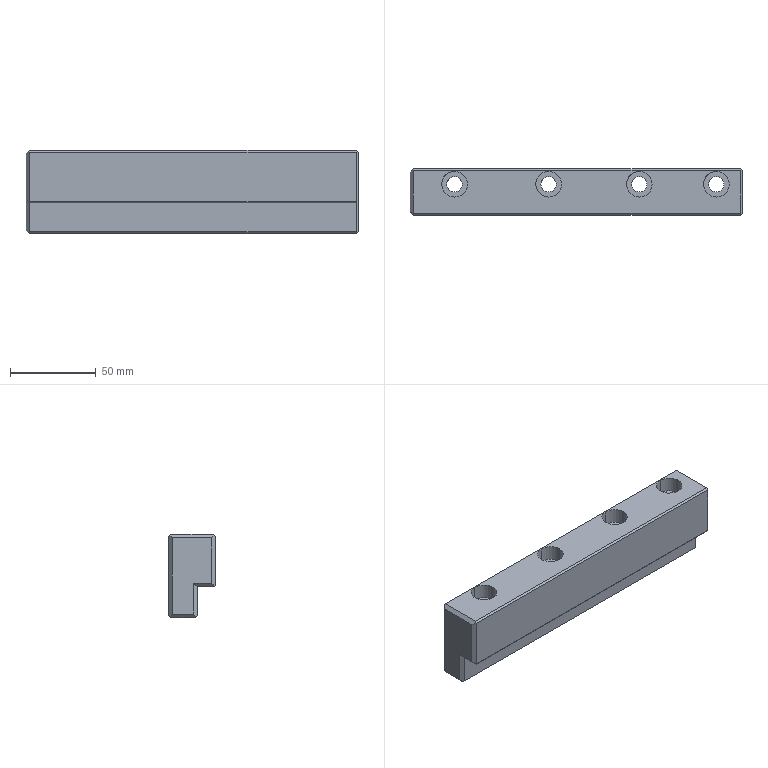Part | Creo | 1 solid | 45 faces | box 194 x 27 x 48.5 mm | volume 200192 mm3 | plane 29 | cylinder 16 | commonest cylinder face diameters 9 x8 15 x8
STEP:
#1=CARTESIAN_POINT('',(-122.,174.995,-41.));
#2=VERTEX_POINT('',#1);
#3=CARTESIAN_POINT('',(-122.,174.995,-12.));
#4=VERTEX_POINT('',#3);
#5=CARTESIAN_POINT('',(-122.,174.995,-41.));
#6=DIRECTION('',(0.,0.,1.));
#7=VECTOR('',#6,29.);
#8=LINE('',#5,#7);
#9=EDGE_CURVE('',#2,#4,#8,.T.);
#10=ORIENTED_EDGE('',*,*,#9,.F.);
#11=CARTESIAN_POINT('',(-313.,174.995,-41.));
#12=VERTEX_POINT('',#11);
#13=CARTESIAN_POINT('',(-313.,174.995,-41.));
#14=DIRECTION('',(1.,0.,0.));
#15=VECTOR('',#14,191.);
#16=LINE('',#13,#15);
#17=EDGE_CURVE('',#12,#2,#16,.T.);
#18=ORIENTED_EDGE('',*,*,#17,.F.);
#19=CARTESIAN_POINT('',(-313.,174.995,-12.));
#20=VERTEX_POINT('',#19);
#21=CARTESIAN_POINT('',(-313.,174.995,-12.));
#22=DIRECTION('',(0.,0.,-1.));
#23=VECTOR('',#22,29.);
#24=LINE('',#21,#23);
#25=EDGE_CURVE('',#20,#12,#24,.T.);
#26=ORIENTED_EDGE('',*,*,#25,.F.);
#27=CARTESIAN_POINT('',(-313.,174.995,-12.));
#28=DIRECTION('',(1.,0.,0.));
#29=VECTOR('',#28,191.);
#30=LINE('',#27,#29);
#31=EDGE_CURVE('',#20,#4,#30,.T.);
#32=ORIENTED_EDGE('',*,*,#31,.T.);
#33=EDGE_LOOP('',(#10,#18,#26,#32));
#34=FACE_OUTER_BOUND('',#33,.F.);
#35=CARTESIAN_POINT('',(-264.,174.995,-8.));
#36=DIRECTION('',(0.,-1.,0.));
#37=DIRECTION('',(0.,0.,1.));
#38=AXIS2_PLACEMENT_3D('',#35,#36,#37);
#39=PLANE('',#38);
#40=ADVANCED_FACE('',(#34),#39,.T.);
#41=CARTESIAN_POINT('',(-121.,175.995,-40.5));
#42=VERTEX_POINT('',#41);
#43=CARTESIAN_POINT('',(-121.,175.995,-12.));
#44=VERTEX_POINT('',#43);
#45=CARTESIAN_POINT('',(-121.,175.995,-40.5));
#46=DIRECTION('',(0.,0.,1.));
#47=VECTOR('',#46,28.5);
#48=LINE('',#45,#47);
#49=EDGE_CURVE('',#42,#44,#48,.T.);
#50=ORIENTED_EDGE('',*,*,#49,.F.);
#51=CARTESIAN_POINT('',(-121.75,175.245,-41.25));
#52=VERTEX_POINT('',#51);
#53=CARTESIAN_POINT('',(-121.,175.995,-40.5));
#54=DIRECTION('',(-0.5774,-0.5774,-0.5774));
#55=VECTOR('',#54,1.299);
#56=LINE('',#53,#55);
#57=EDGE_CURVE('',#42,#52,#56,.T.);
#58=ORIENTED_EDGE('',*,*,#57,.T.);
#59=CARTESIAN_POINT('',(-121.75,175.245,-41.25));
#60=DIRECTION('',(-0.5774,-0.5774,0.5774));
#61=VECTOR('',#60,0.433);
#62=LINE('',#59,#61);
#63=EDGE_CURVE('',#52,#2,#62,.T.);
#64=ORIENTED_EDGE('',*,*,#63,.T.);
#65=ORIENTED_EDGE('',*,*,#9,.T.);
#66=CARTESIAN_POINT('',(-121.5,175.495,-11.5));
#67=VERTEX_POINT('',#66);
#68=CARTESIAN_POINT('',(-122.,174.995,-12.));
#69=DIRECTION('',(0.5774,0.5774,0.5774));
#70=VECTOR('',#69,0.866);
#71=LINE('',#68,#70);
#72=EDGE_CURVE('',#4,#67,#71,.T.);
#73=ORIENTED_EDGE('',*,*,#72,.T.);
#74=CARTESIAN_POINT('',(-121.5,175.495,-11.5));
#75=DIRECTION('',(0.5774,0.5774,-0.5774));
#76=VECTOR('',#75,0.866);
#77=LINE('',#74,#76);
#78=EDGE_CURVE('',#67,#44,#77,.T.);
#79=ORIENTED_EDGE('',*,*,#78,.T.);
#80=EDGE_LOOP('',(#50,#58,#64,#65,#73,#79));
#81=FACE_OUTER_BOUND('',#80,.F.);
#82=CARTESIAN_POINT('',(-121.5,175.495,-25.75));
#83=DIRECTION('',(0.7071,-0.7071,0.));
#84=DIRECTION('',(0.7071,0.7071,0.));
#85=AXIS2_PLACEMENT_3D('',#82,#83,#84);
#86=PLANE('',#85);
#87=ADVANCED_FACE('',(#81),#86,.T.);
#88=CARTESIAN_POINT('',(-121.,200.995,-12.));
#89=VERTEX_POINT('',#88);
#90=CARTESIAN_POINT('',(-121.,200.995,-58.5));
#91=VERTEX_POINT('',#90);
#92=CARTESIAN_POINT('',(-121.,200.995,-12.));
#93=DIRECTION('',(0.,0.,-1.));
#94=VECTOR('',#93,46.5);
#95=LINE('',#92,#94);
#96=EDGE_CURVE('',#89,#91,#95,.T.);
#97=ORIENTED_EDGE('',*,*,#96,.T.);
#98=CARTESIAN_POINT('',(-121.,186.495,-58.5));
#99=VERTEX_POINT('',#98);
#100=CARTESIAN_POINT('',(-121.,200.995,-58.5));
#101=DIRECTION('',(0.,-1.,0.));
#102=VECTOR('',#101,14.5);
#103=LINE('',#100,#102);
#104=EDGE_CURVE('',#91,#99,#103,.T.);
#105=ORIENTED_EDGE('',*,*,#104,.T.);
#106=CARTESIAN_POINT('',(-121.,186.495,-40.5));
#107=VERTEX_POINT('',#106);
#108=CARTESIAN_POINT('',(-121.,186.495,-58.5));
#109=DIRECTION('',(0.,0.,1.));
#110=VECTOR('',#109,18.);
#111=LINE('',#108,#110);
#112=EDGE_CURVE('',#99,#107,#111,.T.);
#113=ORIENTED_EDGE('',*,*,#112,.T.);
#114=CARTESIAN_POINT('',(-121.,186.495,-40.5));
#115=DIRECTION('',(0.,-1.,0.));
#116=VECTOR('',#115,10.5);
#117=LINE('',#114,#116);
#118=EDGE_CURVE('',#107,#42,#117,.T.);
#119=ORIENTED_EDGE('',*,*,#118,.T.);
#120=ORIENTED_EDGE('',*,*,#49,.T.);
#121=CARTESIAN_POINT('',(-121.,175.995,-12.));
#122=DIRECTION('',(0.,1.,0.));
#123=VECTOR('',#122,25.);
#124=LINE('',#121,#123);
#125=EDGE_CURVE('',#44,#89,#124,.T.);
#126=ORIENTED_EDGE('',*,*,#125,.T.);
#127=EDGE_LOOP('',(#97,#105,#113,#119,#120,#126));
#128=FACE_OUTER_BOUND('',#127,.F.);
#129=CARTESIAN_POINT('',(-121.,183.495,-43.5));
#130=DIRECTION('',(1.,0.,0.));
#131=DIRECTION('',(0.,0.,-1.));
#132=AXIS2_PLACEMENT_3D('',#129,#130,#131);
#133=PLANE('',#132);
#134=ADVANCED_FACE('',(#128),#133,.T.);
#135=CARTESIAN_POINT('',(-122.,201.995,-12.));
#136=VERTEX_POINT('',#135);
#137=CARTESIAN_POINT('',(-122.,201.995,-58.5));
#138=VERTEX_POINT('',#137);
#139=CARTESIAN_POINT('',(-122.,201.995,-12.));
#140=DIRECTION('',(0.,0.,-1.));
#141=VECTOR('',#140,46.5);
#142=LINE('',#139,#141);
#143=EDGE_CURVE('',#136,#138,#142,.T.);
#144=ORIENTED_EDGE('',*,*,#143,.T.);
#145=CARTESIAN_POINT('',(-121.5,201.495,-59.));
#146=VERTEX_POINT('',#145);
#147=CARTESIAN_POINT('',(-121.5,201.495,-59.));
#148=DIRECTION('',(-0.5774,0.5774,0.5774));
#149=VECTOR('',#148,0.866);
#150=LINE('',#147,#149);
#151=EDGE_CURVE('',#146,#138,#150,.T.);
#152=ORIENTED_EDGE('',*,*,#151,.F.);
#153=CARTESIAN_POINT('',(-121.,200.995,-58.5));
#154=DIRECTION('',(-0.5774,0.5774,-0.5774));
#155=VECTOR('',#154,0.866);
#156=LINE('',#153,#155);
#157=EDGE_CURVE('',#91,#146,#156,.T.);
#158=ORIENTED_EDGE('',*,*,#157,.F.);
#159=ORIENTED_EDGE('',*,*,#96,.F.);
#160=CARTESIAN_POINT('',(-121.5,201.495,-11.5));
#161=VERTEX_POINT('',#160);
#162=CARTESIAN_POINT('',(-121.,200.995,-12.));
#163=DIRECTION('',(-0.5774,0.5774,0.5774));
#164=VECTOR('',#163,0.866);
#165=LINE('',#162,#164);
#166=EDGE_CURVE('',#89,#161,#165,.T.);
#167=ORIENTED_EDGE('',*,*,#166,.T.);
#168=CARTESIAN_POINT('',(-121.5,201.495,-11.5));
#169=DIRECTION('',(-0.5774,0.5774,-0.5774));
#170=VECTOR('',#169,0.866);
#171=LINE('',#168,#170);
#172=EDGE_CURVE('',#161,#136,#171,.T.);
#173=ORIENTED_EDGE('',*,*,#172,.T.);
#174=EDGE_LOOP('',(#144,#152,#158,#159,#167,#173));
#175=FACE_OUTER_BOUND('',#174,.F.);
#176=CARTESIAN_POINT('',(-121.5,201.495,-33.75));
#177=DIRECTION('',(0.7071,0.7071,0.));
#178=DIRECTION('',(0.7071,-0.7071,0.));
#179=AXIS2_PLACEMENT_3D('',#176,#177,#178);
#180=PLANE('',#179);
#181=ADVANCED_FACE('',(#175),#180,.T.);
#182=CARTESIAN_POINT('',(-313.,201.995,-58.5));
#183=VERTEX_POINT('',#182);
#184=CARTESIAN_POINT('',(-313.,201.995,-12.));
#185=VERTEX_POINT('',#184);
#186=CARTESIAN_POINT('',(-313.,201.995,-58.5));
#187=DIRECTION('',(0.,0.,1.));
#188=VECTOR('',#187,46.5);
#189=LINE('',#186,#188);
#190=EDGE_CURVE('',#183,#185,#189,.T.);
#191=ORIENTED_EDGE('',*,*,#190,.F.);
#192=CARTESIAN_POINT('',(-313.,201.995,-58.5));
#193=DIRECTION('',(1.,0.,0.));
#194=VECTOR('',#193,191.);
#195=LINE('',#192,#194);
#196=EDGE_CURVE('',#183,#138,#195,.T.);
#197=ORIENTED_EDGE('',*,*,#196,.T.);
#198=ORIENTED_EDGE('',*,*,#143,.F.);
#199=CARTESIAN_POINT('',(-122.,201.995,-12.));
#200=DIRECTION('',(-1.,0.,0.));
#201=VECTOR('',#200,191.);
#202=LINE('',#199,#201);
#203=EDGE_CURVE('',#136,#185,#202,.T.);
#204=ORIENTED_EDGE('',*,*,#203,.T.);
#205=EDGE_LOOP('',(#191,#197,#198,#204));
#206=FACE_OUTER_BOUND('',#205,.F.);
#207=CARTESIAN_POINT('',(-264.,201.995,-59.5));
#208=DIRECTION('',(0.,1.,0.));
#209=DIRECTION('',(0.,0.,-1.));
#210=AXIS2_PLACEMENT_3D('',#207,#208,#209);
#211=PLANE('',#210);
#212=ADVANCED_FACE('',(#206),#211,.T.);
#213=CARTESIAN_POINT('',(-315.,199.995,-57.5));
#214=VERTEX_POINT('',#213);
#215=CARTESIAN_POINT('',(-315.,199.995,-13.));
#216=VERTEX_POINT('',#215);
#217=CARTESIAN_POINT('',(-315.,199.995,-57.5));
#218=DIRECTION('',(0.,0.,1.));
#219=VECTOR('',#218,44.5);
#220=LINE('',#217,#219);
#221=EDGE_CURVE('',#214,#216,#220,.T.);
#222=ORIENTED_EDGE('',*,*,#221,.F.);
#223=CARTESIAN_POINT('',(-313.5,201.495,-59.));
#224=VERTEX_POINT('',#223);
#225=CARTESIAN_POINT('',(-313.5,201.495,-59.));
#226=DIRECTION('',(-0.5774,-0.5774,0.5774));
#227=VECTOR('',#226,2.598);
#228=LINE('',#225,#227);
#229=EDGE_CURVE('',#224,#214,#228,.T.);
#230=ORIENTED_EDGE('',*,*,#229,.F.);
#231=CARTESIAN_POINT('',(-313.,201.995,-58.5));
#232=DIRECTION('',(-0.5774,-0.5774,-0.5774));
#233=VECTOR('',#232,0.866);
#234=LINE('',#231,#233);
#235=EDGE_CURVE('',#183,#224,#234,.T.);
#236=ORIENTED_EDGE('',*,*,#235,.F.);
#237=ORIENTED_EDGE('',*,*,#190,.T.);
#238=CARTESIAN_POINT('',(-313.5,201.495,-11.5));
#239=VERTEX_POINT('',#238);
#240=CARTESIAN_POINT('',(-313.,201.995,-12.));
#241=DIRECTION('',(-0.5774,-0.5774,0.5774));
#242=VECTOR('',#241,0.866);
#243=LINE('',#240,#242);
#244=EDGE_CURVE('',#185,#239,#243,.T.);
#245=ORIENTED_EDGE('',*,*,#244,.T.);
#246=CARTESIAN_POINT('',(-313.5,201.495,-11.5));
#247=DIRECTION('',(-0.5774,-0.5774,-0.5774));
#248=VECTOR('',#247,2.598);
#249=LINE('',#246,#248);
#250=EDGE_CURVE('',#239,#216,#249,.T.);
#251=ORIENTED_EDGE('',*,*,#250,.T.);
#252=EDGE_LOOP('',(#222,#230,#236,#237,#245,#251));
#253=FACE_OUTER_BOUND('',#252,.F.);
#254=CARTESIAN_POINT('',(-313.5,201.495,-33.75));
#255=DIRECTION('',(-0.7071,0.7071,0.));
#256=DIRECTION('',(-0.7071,-0.7071,0.));
#257=AXIS2_PLACEMENT_3D('',#254,#255,#256);
#258=PLANE('',#257);
#259=ADVANCED_FACE('',(#253),#258,.T.);
#260=CARTESIAN_POINT('',(-315.,176.995,-13.));
#261=VERTEX_POINT('',#260);
#262=CARTESIAN_POINT('',(-315.,176.995,-39.5));
#263=VERTEX_POINT('',#262);
#264=CARTESIAN_POINT('',(-315.,176.995,-13.));
#265=DIRECTION('',(0.,0.,-1.));
#266=VECTOR('',#265,26.5);
#267=LINE('',#264,#266);
#268=EDGE_CURVE('',#261,#263,#267,.T.);
#269=ORIENTED_EDGE('',*,*,#268,.T.);
#270=CARTESIAN_POINT('',(-315.,187.495,-39.5));
#271=VERTEX_POINT('',#270);
#272=CARTESIAN_POINT('',(-315.,176.995,-39.5));
#273=DIRECTION('',(0.,1.,0.));
#274=VECTOR('',#273,10.5);
#275=LINE('',#272,#274);
#276=EDGE_CURVE('',#263,#271,#275,.T.);
#277=ORIENTED_EDGE('',*,*,#276,.T.);
#278=CARTESIAN_POINT('',(-315.,187.495,-57.5));
#279=VERTEX_POINT('',#278);
#280=CARTESIAN_POINT('',(-315.,187.495,-39.5));
#281=DIRECTION('',(0.,0.,-1.));
#282=VECTOR('',#281,18.);
#283=LINE('',#280,#282);
#284=EDGE_CURVE('',#271,#279,#283,.T.);
#285=ORIENTED_EDGE('',*,*,#284,.T.);
#286=CARTESIAN_POINT('',(-315.,187.495,-57.5));
#287=DIRECTION('',(0.,1.,0.));
#288=VECTOR('',#287,12.5);
#289=LINE('',#286,#288);
#290=EDGE_CURVE('',#279,#214,#289,.T.);
#291=ORIENTED_EDGE('',*,*,#290,.T.);
#292=ORIENTED_EDGE('',*,*,#221,.T.);
#293=CARTESIAN_POINT('',(-315.,199.995,-13.));
#294=DIRECTION('',(0.,-1.,0.));
#295=VECTOR('',#294,23.);
#296=LINE('',#293,#295);
#297=EDGE_CURVE('',#216,#261,#296,.T.);
#298=ORIENTED_EDGE('',*,*,#297,.T.);
#299=EDGE_LOOP('',(#269,#277,#285,#291,#292,#298));
#300=FACE_OUTER_BOUND('',#299,.F.);
#301=CARTESIAN_POINT('',(-315.,-0.004699,-11.));
#302=DIRECTION('',(1.,0.,0.));
#303=DIRECTION('',(0.,1.,0.));
#304=AXIS2_PLACEMENT_3D('',#301,#302,#303);
#305=PLANE('',#304);
#306=ADVANCED_FACE('',(#300),#305,.F.);
#307=CARTESIAN_POINT('',(-313.5,175.495,-11.5));
#308=VERTEX_POINT('',#307);
#309=CARTESIAN_POINT('',(-313.5,175.495,-11.5));
#310=DIRECTION('',(0.5774,-0.5774,-0.5774));
#311=VECTOR('',#310,0.866);
#312=LINE('',#309,#311);
#313=EDGE_CURVE('',#308,#20,#312,.T.);
#314=ORIENTED_EDGE('',*,*,#313,.T.);
#315=ORIENTED_EDGE('',*,*,#25,.T.);
#316=CARTESIAN_POINT('',(-313.25,175.245,-41.25));
#317=VERTEX_POINT('',#316);
#318=CARTESIAN_POINT('',(-313.,174.995,-41.));
#319=DIRECTION('',(-0.5774,0.5774,-0.5774));
#320=VECTOR('',#319,0.433);
#321=LINE('',#318,#320);
#322=EDGE_CURVE('',#12,#317,#321,.T.);
#323=ORIENTED_EDGE('',*,*,#322,.T.);
#324=CARTESIAN_POINT('',(-315.,176.995,-39.5));
#325=DIRECTION('',(0.5774,-0.5774,-0.5774));
#326=VECTOR('',#325,3.031);
#327=LINE('',#324,#326);
#328=EDGE_CURVE('',#263,#317,#327,.T.);
#329=ORIENTED_EDGE('',*,*,#328,.F.);
#330=ORIENTED_EDGE('',*,*,#268,.F.);
#331=CARTESIAN_POINT('',(-315.,176.995,-13.));
#332=DIRECTION('',(0.5774,-0.5774,0.5774));
#333=VECTOR('',#332,2.598);
#334=LINE('',#331,#333);
#335=EDGE_CURVE('',#261,#308,#334,.T.);
#336=ORIENTED_EDGE('',*,*,#335,.T.);
#337=EDGE_LOOP('',(#314,#315,#323,#329,#330,#336));
#338=FACE_OUTER_BOUND('',#337,.F.);
#339=CARTESIAN_POINT('',(-313.5,175.495,-25.75));
#340=DIRECTION('',(-0.7071,-0.7071,0.));
#341=DIRECTION('',(-0.7071,0.7071,0.));
#342=AXIS2_PLACEMENT_3D('',#339,#340,#341);
#343=PLANE('',#342);
#344=ADVANCED_FACE('',(#338),#343,.T.);
#345=CARTESIAN_POINT('',(-122.,175.995,-11.));
#346=VERTEX_POINT('',#345);
#347=CARTESIAN_POINT('',(-122.,175.995,-11.));
#348=DIRECTION('',(0.5774,-0.5774,-0.5774));
#349=VECTOR('',#348,0.866);
#350=LINE('',#347,#349);
#351=EDGE_CURVE('',#346,#67,#350,.T.);
#352=ORIENTED_EDGE('',*,*,#351,.T.);
#353=ORIENTED_EDGE('',*,*,#72,.F.);
#354=ORIENTED_EDGE('',*,*,#31,.F.);
#355=ORIENTED_EDGE('',*,*,#313,.F.);
#356=CARTESIAN_POINT('',(-313.,175.995,-11.));
#357=VERTEX_POINT('',#356);
#358=CARTESIAN_POINT('',(-313.,175.995,-11.));
#359=DIRECTION('',(-0.5774,-0.5774,-0.5774));
#360=VECTOR('',#359,0.866);
#361=LINE('',#358,#360);
#362=EDGE_CURVE('',#357,#308,#361,.T.);
#363=ORIENTED_EDGE('',*,*,#362,.F.);
#364=CARTESIAN_POINT('',(-122.,175.995,-11.));
#365=DIRECTION('',(-1.,0.,0.));
#366=VECTOR('',#365,191.);
#367=LINE('',#364,#366);
#368=EDGE_CURVE('',#346,#357,#367,.T.);
#369=ORIENTED_EDGE('',*,*,#368,.F.);
#370=EDGE_LOOP('',(#352,#353,#354,#355,#363,#369));
#371=FACE_OUTER_BOUND('',#370,.F.);
#372=CARTESIAN_POINT('',(-264.,174.995,-12.));
#373=DIRECTION('',(0.,0.7071,-0.7071));
#374=DIRECTION('',(-1.,0.,0.));
#375=AXIS2_PLACEMENT_3D('',#372,#373,#374);
#376=PLANE('',#375);
#377=ADVANCED_FACE('',(#371),#376,.F.);
#378=CARTESIAN_POINT('',(-122.,200.995,-11.));
#379=VERTEX_POINT('',#378);
#380=CARTESIAN_POINT('',(-121.5,201.495,-11.5));
#381=DIRECTION('',(-0.5774,-0.5774,0.5774));
#382=VECTOR('',#381,0.866);
#383=LINE('',#380,#382);
#384=EDGE_CURVE('',#161,#379,#383,.T.);
#385=ORIENTED_EDGE('',*,*,#384,.F.);
#386=ORIENTED_EDGE('',*,*,#166,.F.);
#387=ORIENTED_EDGE('',*,*,#125,.F.);
#388=ORIENTED_EDGE('',*,*,#78,.F.);
#389=ORIENTED_EDGE('',*,*,#351,.F.);
#390=CARTESIAN_POINT('',(-122.,200.995,-11.));
#391=DIRECTION('',(0.,-1.,0.));
#392=VECTOR('',#391,25.);
#393=LINE('',#390,#392);
#394=EDGE_CURVE('',#379,#346,#393,.T.);
#395=ORIENTED_EDGE('',*,*,#394,.F.);
#396=EDGE_LOOP('',(#385,#386,#387,#388,#389,#395));
#397=FACE_OUTER_BOUND('',#396,.F.);
#398=CARTESIAN_POINT('',(-121.,183.495,-12.));
#399=DIRECTION('',(-0.7071,0.,-0.7071));
#400=DIRECTION('',(0.,-1.,0.));
#401=AXIS2_PLACEMENT_3D('',#398,#399,#400);
#402=PLANE('',#401);
#403=ADVANCED_FACE('',(#397),#402,.F.);
#404=ORIENTED_EDGE('',*,*,#203,.F.);
#405=ORIENTED_EDGE('',*,*,#172,.F.);
#406=ORIENTED_EDGE('',*,*,#384,.T.);
#407=CARTESIAN_POINT('',(-313.,200.995,-11.));
#408=VERTEX_POINT('',#407);
#409=CARTESIAN_POINT('',(-313.,200.995,-11.));
#410=DIRECTION('',(1.,0.,0.));
#411=VECTOR('',#410,191.);
#412=LINE('',#409,#411);
#413=EDGE_CURVE('',#408,#379,#412,.T.);
#414=ORIENTED_EDGE('',*,*,#413,.F.);
#415=CARTESIAN_POINT('',(-313.5,201.495,-11.5));
#416=DIRECTION('',(0.5774,-0.5774,0.5774));
#417=VECTOR('',#416,0.866);
#418=LINE('',#415,#417);
#419=EDGE_CURVE('',#239,#408,#418,.T.);
#420=ORIENTED_EDGE('',*,*,#419,.F.);
#421=ORIENTED_EDGE('',*,*,#244,.F.);
#422=EDGE_LOOP('',(#404,#405,#406,#414,#420,#421));
#423=FACE_OUTER_BOUND('',#422,.F.);
#424=CARTESIAN_POINT('',(-265.,200.995,-11.));
#425=DIRECTION('',(0.,-0.7071,-0.7071));
#426=DIRECTION('',(-1.,0.,0.));
#427=AXIS2_PLACEMENT_3D('',#424,#425,#426);
#428=PLANE('',#427);
#429=ADVANCED_FACE('',(#423),#428,.F.);
#430=ORIENTED_EDGE('',*,*,#413,.T.);
#431=ORIENTED_EDGE('',*,*,#394,.T.);
#432=ORIENTED_EDGE('',*,*,#368,.T.);
#433=CARTESIAN_POINT('',(-313.,175.995,-11.));
#434=DIRECTION('',(0.,1.,0.));
#435=VECTOR('',#434,25.);
#436=LINE('',#433,#435);
#437=EDGE_CURVE('',#357,#408,#436,.T.);
#438=ORIENTED_EDGE('',*,*,#437,.T.);
#439=EDGE_LOOP('',(#430,#431,#432,#438));
#440=FACE_OUTER_BOUND('',#439,.F.);
#441=CARTESIAN_POINT('',(-128.5,192.995,-11.));
#442=VERTEX_POINT('',#441);
#443=CARTESIAN_POINT('',(-136.,185.495,-11.));
#444=VERTEX_POINT('',#443);
#445=CARTESIAN_POINT('',(-136.,192.995,-11.));
#446=DIRECTION('',(0.,0.,-1.));
#447=DIRECTION('',(1.,0.,0.));
#448=AXIS2_PLACEMENT_3D('',#445,#446,#447);
#449=CIRCLE('',#448,7.5);
#450=EDGE_CURVE('',#442,#444,#449,.T.);
#451=ORIENTED_EDGE('',*,*,#450,.F.);
#452=CARTESIAN_POINT('',(-136.,200.495,-11.));
#453=VERTEX_POINT('',#452);
#454=CARTESIAN_POINT('',(-136.,192.995,-11.));
#455=DIRECTION('',(0.,0.,-1.));
#456=DIRECTION('',(0.,1.,0.));
#457=AXIS2_PLACEMENT_3D('',#454,#455,#456);
#458=CIRCLE('',#457,7.5);
#459=EDGE_CURVE('',#453,#442,#458,.T.);
#460=ORIENTED_EDGE('',*,*,#459,.F.);
#461=CARTESIAN_POINT('',(-136.,192.995,-11.));
#462=DIRECTION('',(0.,0.,-1.));
#463=DIRECTION('',(0.,-1.,0.));
#464=AXIS2_PLACEMENT_3D('',#461,#462,#463);
#465=CIRCLE('',#464,7.5);
#466=EDGE_CURVE('',#444,#453,#465,.T.);
#467=ORIENTED_EDGE('',*,*,#466,.F.);
#468=EDGE_LOOP('',(#451,#460,#467));
#469=FACE_BOUND('',#468,.F.);
#470=CARTESIAN_POINT('',(-173.5,192.995,-11.));
#471=VERTEX_POINT('',#470);
#472=CARTESIAN_POINT('',(-181.,185.495,-11.));
#473=VERTEX_POINT('',#472);
#474=CARTESIAN_POINT('',(-181.,192.995,-11.));
#475=DIRECTION('',(0.,0.,-1.));
#476=DIRECTION('',(1.,0.,0.));
#477=AXIS2_PLACEMENT_3D('',#474,#475,#476);
#478=CIRCLE('',#477,7.5);
#479=EDGE_CURVE('',#471,#473,#478,.T.);
#480=ORIENTED_EDGE('',*,*,#479,.F.);
#481=CARTESIAN_POINT('',(-181.,200.495,-11.));
#482=VERTEX_POINT('',#481);
#483=CARTESIAN_POINT('',(-181.,192.995,-11.));
#484=DIRECTION('',(0.,0.,-1.));
#485=DIRECTION('',(0.,1.,0.));
#486=AXIS2_PLACEMENT_3D('',#483,#484,#485);
#487=CIRCLE('',#486,7.5);
#488=EDGE_CURVE('',#482,#471,#487,.T.);
#489=ORIENTED_EDGE('',*,*,#488,.F.);
#490=CARTESIAN_POINT('',(-181.,192.995,-11.));
#491=DIRECTION('',(0.,0.,-1.));
#492=DIRECTION('',(0.,-1.,0.));
#493=AXIS2_PLACEMENT_3D('',#490,#491,#492);
#494=CIRCLE('',#493,7.5);
#495=EDGE_CURVE('',#473,#482,#494,.T.);
#496=ORIENTED_EDGE('',*,*,#495,.F.);
#497=EDGE_LOOP('',(#480,#489,#496));
#498=FACE_BOUND('',#497,.F.);
#499=CARTESIAN_POINT('',(-281.5,192.995,-11.));
#500=VERTEX_POINT('',#499);
#501=CARTESIAN_POINT('',(-289.,185.495,-11.));
#502=VERTEX_POINT('',#501);
#503=CARTESIAN_POINT('',(-289.,192.995,-11.));
#504=DIRECTION('',(0.,0.,-1.));
#505=DIRECTION('',(1.,0.,0.));
#506=AXIS2_PLACEMENT_3D('',#503,#504,#505);
#507=CIRCLE('',#506,7.5);
#508=EDGE_CURVE('',#500,#502,#507,.T.);
#509=ORIENTED_EDGE('',*,*,#508,.F.);
#510=CARTESIAN_POINT('',(-289.,200.495,-11.));
#511=VERTEX_POINT('',#510);
#512=CARTESIAN_POINT('',(-289.,192.995,-11.));
#513=DIRECTION('',(0.,0.,-1.));
#514=DIRECTION('',(0.,1.,0.));
#515=AXIS2_PLACEMENT_3D('',#512,#513,#514);
#516=CIRCLE('',#515,7.5);
#517=EDGE_CURVE('',#511,#500,#516,.T.);
#518=ORIENTED_EDGE('',*,*,#517,.F.);
#519=CARTESIAN_POINT('',(-289.,192.995,-11.));
#520=DIRECTION('',(0.,0.,-1.));
#521=DIRECTION('',(0.,-1.,0.));
#522=AXIS2_PLACEMENT_3D('',#519,#520,#521);
#523=CIRCLE('',#522,7.5);
#524=EDGE_CURVE('',#502,#511,#523,.T.);
#525=ORIENTED_EDGE('',*,*,#524,.F.);
#526=EDGE_LOOP('',(#509,#518,#525));
#527=FACE_BOUND('',#526,.F.);
#528=CARTESIAN_POINT('',(-226.5,192.995,-11.));
#529=VERTEX_POINT('',#528);
#530=CARTESIAN_POINT('',(-234.,185.495,-11.));
#531=VERTEX_POINT('',#530);
#532=CARTESIAN_POINT('',(-234.,192.995,-11.));
#533=DIRECTION('',(0.,0.,-1.));
#534=DIRECTION('',(1.,0.,0.));
#535=AXIS2_PLACEMENT_3D('',#532,#533,#534);
#536=CIRCLE('',#535,7.5);
#537=EDGE_CURVE('',#529,#531,#536,.T.);
#538=ORIENTED_EDGE('',*,*,#537,.F.);
#539=CARTESIAN_POINT('',(-234.,200.495,-11.));
#540=VERTEX_POINT('',#539);
#541=CARTESIAN_POINT('',(-234.,192.995,-11.));
#542=DIRECTION('',(0.,0.,-1.));
#543=DIRECTION('',(0.,1.,0.));
#544=AXIS2_PLACEMENT_3D('',#541,#542,#543);
#545=CIRCLE('',#544,7.5);
#546=EDGE_CURVE('',#540,#529,#545,.T.);
#547=ORIENTED_EDGE('',*,*,#546,.F.);
#548=CARTESIAN_POINT('',(-234.,192.995,-11.));
#549=DIRECTION('',(0.,0.,-1.));
#550=DIRECTION('',(0.,-1.,0.));
#551=AXIS2_PLACEMENT_3D('',#548,#549,#550);
#552=CIRCLE('',#551,7.5);
#553=EDGE_CURVE('',#531,#540,#552,.T.);
#554=ORIENTED_EDGE('',*,*,#553,.F.);
#555=EDGE_LOOP('',(#538,#547,#554));
#556=FACE_BOUND('',#555,.F.);
#557=CARTESIAN_POINT('',(-265.,347.995,-11.));
#558=DIRECTION('',(0.,0.,1.));
#559=DIRECTION('',(0.,-1.,0.));
#560=AXIS2_PLACEMENT_3D('',#557,#558,#559);
#561=PLANE('',#560);
#562=ADVANCED_FACE('',(#440,#469,#498,#527,#556),#561,.T.);
#563=ORIENTED_EDGE('',*,*,#362,.T.);
#564=ORIENTED_EDGE('',*,*,#335,.F.);
#565=ORIENTED_EDGE('',*,*,#297,.F.);
#566=ORIENTED_EDGE('',*,*,#250,.F.);
#567=ORIENTED_EDGE('',*,*,#419,.T.);
#568=ORIENTED_EDGE('',*,*,#437,.F.);
#569=EDGE_LOOP('',(#563,#564,#565,#566,#567,#568));
#570=FACE_OUTER_BOUND('',#569,.F.);
#571=CARTESIAN_POINT('',(-314.,183.495,-12.));
#572=DIRECTION('',(-0.7071,0.,0.7071));
#573=DIRECTION('',(0.,-1.,0.));
#574=AXIS2_PLACEMENT_3D('',#571,#572,#573);
#575=PLANE('',#574);
#576=ADVANCED_FACE('',(#570),#575,.T.);
#577=ORIENTED_EDGE('',*,*,#459,.T.);
#578=ORIENTED_EDGE('',*,*,#450,.T.);
#579=CARTESIAN_POINT('',(-136.,185.495,-20.));
#580=VERTEX_POINT('',#579);
#581=CARTESIAN_POINT('',(-136.,185.495,-11.));
#582=DIRECTION('',(0.,0.,-1.));
#583=VECTOR('',#582,9.);
#584=LINE('',#581,#583);
#585=EDGE_CURVE('',#444,#580,#584,.T.);
#586=ORIENTED_EDGE('',*,*,#585,.T.);
#587=CARTESIAN_POINT('',(-128.5,192.995,-20.));
#588=VERTEX_POINT('',#587);
#589=CARTESIAN_POINT('',(-136.,192.995,-20.));
#590=DIRECTION('',(0.,0.,1.));
#591=DIRECTION('',(0.,-1.,0.));
#592=AXIS2_PLACEMENT_3D('',#589,#590,#591);
#593=CIRCLE('',#592,7.5);
#594=EDGE_CURVE('',#580,#588,#593,.T.);
#595=ORIENTED_EDGE('',*,*,#594,.T.);
#596=CARTESIAN_POINT('',(-136.,200.495,-20.));
#597=VERTEX_POINT('',#596);
#598=CARTESIAN_POINT('',(-136.,192.995,-20.));
#599=DIRECTION('',(0.,0.,1.));
#600=DIRECTION('',(1.,0.,0.));
#601=AXIS2_PLACEMENT_3D('',#598,#599,#600);
#602=CIRCLE('',#601,7.5);
#603=EDGE_CURVE('',#588,#597,#602,.T.);
#604=ORIENTED_EDGE('',*,*,#603,.T.);
#605=CARTESIAN_POINT('',(-136.,200.495,-11.));
#606=DIRECTION('',(0.,0.,-1.));
#607=VECTOR('',#606,9.);
#608=LINE('',#605,#607);
#609=EDGE_CURVE('',#453,#597,#608,.T.);
#610=ORIENTED_EDGE('',*,*,#609,.F.);
#611=EDGE_LOOP('',(#577,#578,#586,#595,#604,#610));
#612=FACE_OUTER_BOUND('',#611,.F.);
#613=CARTESIAN_POINT('',(-136.,192.995,-17.55));
#614=DIRECTION('',(0.,0.,-1.));
#615=DIRECTION('',(0.,-1.,0.));
#616=AXIS2_PLACEMENT_3D('',#613,#614,#615);
#617=CYLINDRICAL_SURFACE('',#616,7.5);
#618=ADVANCED_FACE('',(#612),#617,.F.);
#619=ORIENTED_EDGE('',*,*,#466,.T.);
#620=ORIENTED_EDGE('',*,*,#609,.T.);
#621=CARTESIAN_POINT('',(-143.5,192.995,-20.));
#622=VERTEX_POINT('',#621);
#623=CARTESIAN_POINT('',(-136.,192.995,-20.));
#624=DIRECTION('',(0.,0.,1.));
#625=DIRECTION('',(0.,1.,0.));
#626=AXIS2_PLACEMENT_3D('',#623,#624,#625);
#627=CIRCLE('',#626,7.5);
#628=EDGE_CURVE('',#597,#622,#627,.T.);
#629=ORIENTED_EDGE('',*,*,#628,.T.);
#630=CARTESIAN_POINT('',(-136.,192.995,-20.));
#631=DIRECTION('',(0.,0.,1.));
#632=DIRECTION('',(-1.,0.,0.));
#633=AXIS2_PLACEMENT_3D('',#630,#631,#632);
#634=CIRCLE('',#633,7.5);
#635=EDGE_CURVE('',#622,#580,#634,.T.);
#636=ORIENTED_EDGE('',*,*,#635,.T.);
#637=ORIENTED_EDGE('',*,*,#585,.F.);
#638=EDGE_LOOP('',(#619,#620,#629,#636,#637));
#639=FACE_OUTER_BOUND('',#638,.F.);
#640=CARTESIAN_POINT('',(-136.,192.995,-17.55));
#641=DIRECTION('',(0.,0.,-1.));
#642=DIRECTION('',(0.,-1.,0.));
#643=AXIS2_PLACEMENT_3D('',#640,#641,#642);
#644=CYLINDRICAL_SURFACE('',#643,7.5);
#645=ADVANCED_FACE('',(#639),#644,.F.);
#646=ORIENTED_EDGE('',*,*,#635,.F.);
#647=ORIENTED_EDGE('',*,*,#628,.F.);
#648=ORIENTED_EDGE('',*,*,#603,.F.);
#649=ORIENTED_EDGE('',*,*,#594,.F.);
#650=EDGE_LOOP('',(#646,#647,#648,#649));
#651=FACE_OUTER_BOUND('',#650,.F.);
#652=CARTESIAN_POINT('',(-140.5,192.995,-20.));
#653=VERTEX_POINT('',#652);
#654=CARTESIAN_POINT('',(-136.,197.495,-20.));
#655=VERTEX_POINT('',#654);
#656=CARTESIAN_POINT('',(-136.,192.995,-20.));
#657=DIRECTION('',(0.,0.,-1.));
#658=DIRECTION('',(-1.,0.,0.));
#659=AXIS2_PLACEMENT_3D('',#656,#657,#658);
#660=CIRCLE('',#659,4.5);
#661=EDGE_CURVE('',#653,#655,#660,.T.);
#662=ORIENTED_EDGE('',*,*,#661,.F.);
#663=CARTESIAN_POINT('',(-136.,188.495,-20.));
#664=VERTEX_POINT('',#663);
#665=CARTESIAN_POINT('',(-136.,192.995,-20.));
#666=DIRECTION('',(0.,0.,-1.));
#667=DIRECTION('',(0.,-1.,0.));
#668=AXIS2_PLACEMENT_3D('',#665,#666,#667);
#669=CIRCLE('',#668,4.5);
#670=EDGE_CURVE('',#664,#653,#669,.T.);
#671=ORIENTED_EDGE('',*,*,#670,.F.);
#672=CARTESIAN_POINT('',(-136.,192.995,-20.));
#673=DIRECTION('',(0.,0.,-1.));
#674=DIRECTION('',(0.,1.,0.));
#675=AXIS2_PLACEMENT_3D('',#672,#673,#674);
#676=CIRCLE('',#675,4.5);
#677=EDGE_CURVE('',#655,#664,#676,.T.);
#678=ORIENTED_EDGE('',*,*,#677,.F.);
#679=EDGE_LOOP('',(#662,#671,#678));
#680=FACE_BOUND('',#679,.F.);
#681=CARTESIAN_POINT('',(-136.,192.995,-20.));
#682=DIRECTION('',(0.,0.,-1.));
#683=DIRECTION('',(0.,-1.,0.));
#684=AXIS2_PLACEMENT_3D('',#681,#682,#683);
#685=PLANE('',#684);
#686=ADVANCED_FACE('',(#651,#680),#685,.F.);
#687=ORIENTED_EDGE('',*,*,#670,.T.);
#688=ORIENTED_EDGE('',*,*,#661,.T.);
#689=CARTESIAN_POINT('',(-136.,197.495,-59.5));
#690=VERTEX_POINT('',#689);
#691=CARTESIAN_POINT('',(-136.,197.495,-59.5));
#692=DIRECTION('',(0.,0.,1.));
#693=VECTOR('',#692,39.5);
#694=LINE('',#691,#693);
#695=EDGE_CURVE('',#690,#655,#694,.T.);
#696=ORIENTED_EDGE('',*,*,#695,.F.);
#697=CARTESIAN_POINT('',(-136.,188.495,-59.5));
#698=VERTEX_POINT('',#697);
#699=CARTESIAN_POINT('',(-136.,192.995,-59.5));
#700=DIRECTION('',(0.,0.,1.));
#701=DIRECTION('',(0.,1.,0.));
#702=AXIS2_PLACEMENT_3D('',#699,#700,#701);
#703=CIRCLE('',#702,4.5);
#704=EDGE_CURVE('',#690,#698,#703,.T.);
#705=ORIENTED_EDGE('',*,*,#704,.T.);
#706=CARTESIAN_POINT('',(-136.,188.495,-59.5));
#707=DIRECTION('',(0.,0.,1.));
#708=VECTOR('',#707,39.5);
#709=LINE('',#706,#708);
#710=EDGE_CURVE('',#698,#664,#709,.T.);
#711=ORIENTED_EDGE('',*,*,#710,.T.);
#712=EDGE_LOOP('',(#687,#688,#696,#705,#711));
#713=FACE_OUTER_BOUND('',#712,.F.);
#714=CARTESIAN_POINT('',(-136.,192.995,-17.));
#715=DIRECTION('',(0.,0.,1.));
#716=DIRECTION('',(0.,-1.,0.));
#717=AXIS2_PLACEMENT_3D('',#714,#715,#716);
#718=CYLINDRICAL_SURFACE('',#717,4.5);
#719=ADVANCED_FACE('',(#713),#718,.F.);
#720=ORIENTED_EDGE('',*,*,#677,.T.);
#721=ORIENTED_EDGE('',*,*,#710,.F.);
#722=CARTESIAN_POINT('',(-136.,192.995,-59.5));
#723=DIRECTION('',(0.,0.,1.));
#724=DIRECTION('',(0.,-1.,0.));
#725=AXIS2_PLACEMENT_3D('',#722,#723,#724);
#726=CIRCLE('',#725,4.5);
#727=EDGE_CURVE('',#698,#690,#726,.T.);
#728=ORIENTED_EDGE('',*,*,#727,.T.);
#729=ORIENTED_EDGE('',*,*,#695,.T.);
#730=EDGE_LOOP('',(#720,#721,#728,#729));
#731=FACE_OUTER_BOUND('',#730,.F.);
#732=CARTESIAN_POINT('',(-136.,192.995,-17.));
#733=DIRECTION('',(0.,0.,1.));
#734=DIRECTION('',(0.,-1.,0.));
#735=AXIS2_PLACEMENT_3D('',#732,#733,#734);
#736=CYLINDRICAL_SURFACE('',#735,4.5);
#737=ADVANCED_FACE('',(#731),#736,.F.);
#738=CARTESIAN_POINT('',(-313.,186.495,-59.5));
#739=VERTEX_POINT('',#738);
#740=CARTESIAN_POINT('',(-313.,200.995,-59.5));
#741=VERTEX_POINT('',#740);
#742=CARTESIAN_POINT('',(-313.,186.495,-59.5));
#743=DIRECTION('',(0.,1.,0.));
#744=VECTOR('',#743,14.5);
#745=LINE('',#742,#744);
#746=EDGE_CURVE('',#739,#741,#745,.T.);
#747=ORIENTED_EDGE('',*,*,#746,.F.);
#748=CARTESIAN_POINT('',(-122.,186.495,-59.5));
#749=VERTEX_POINT('',#748);
#750=CARTESIAN_POINT('',(-313.,186.495,-59.5));
#751=DIRECTION('',(1.,0.,0.));
#752=VECTOR('',#751,191.);
#753=LINE('',#750,#752);
#754=EDGE_CURVE('',#739,#749,#753,.T.);
#755=ORIENTED_EDGE('',*,*,#754,.T.);
#756=CARTESIAN_POINT('',(-122.,200.995,-59.5));
#757=VERTEX_POINT('',#756);
#758=CARTESIAN_POINT('',(-122.,200.995,-59.5));
#759=DIRECTION('',(0.,-1.,0.));
#760=VECTOR('',#759,14.5);
#761=LINE('',#758,#760);
#762=EDGE_CURVE('',#757,#749,#761,.T.);
#763=ORIENTED_EDGE('',*,*,#762,.F.);
#764=CARTESIAN_POINT('',(-313.,200.995,-59.5));
#765=DIRECTION('',(1.,0.,0.));
#766=VECTOR('',#765,191.);
#767=LINE('',#764,#766);
#768=EDGE_CURVE('',#741,#757,#767,.T.);
#769=ORIENTED_EDGE('',*,*,#768,.F.);
#770=EDGE_LOOP('',(#747,#755,#763,#769));
#771=FACE_OUTER_BOUND('',#770,.F.);
#772=CARTESIAN_POINT('',(-234.,197.495,-59.5));
#773=VERTEX_POINT('',#772);
#774=CARTESIAN_POINT('',(-234.,188.495,-59.5));
#775=VERTEX_POINT('',#774);
#776=CARTESIAN_POINT('',(-234.,192.995,-59.5));
#777=DIRECTION('',(0.,0.,1.));
#778=DIRECTION('',(0.,1.,0.));
#779=AXIS2_PLACEMENT_3D('',#776,#777,#778);
#780=CIRCLE('',#779,4.5);
#781=EDGE_CURVE('',#773,#775,#780,.T.);
#782=ORIENTED_EDGE('',*,*,#781,.F.);
#783=CARTESIAN_POINT('',(-234.,192.995,-59.5));
#784=DIRECTION('',(0.,0.,1.));
#785=DIRECTION('',(0.,-1.,0.));
#786=AXIS2_PLACEMENT_3D('',#783,#784,#785);
#787=CIRCLE('',#786,4.5);
#788=EDGE_CURVE('',#775,#773,#787,.T.);
#789=ORIENTED_EDGE('',*,*,#788,.F.);
#790=EDGE_LOOP('',(#782,#789));
#791=FACE_BOUND('',#790,.F.);
#792=CARTESIAN_POINT('',(-289.,197.495,-59.5));
#793=VERTEX_POINT('',#792);
#794=CARTESIAN_POINT('',(-289.,188.495,-59.5));
#795=VERTEX_POINT('',#794);
#796=CARTESIAN_POINT('',(-289.,192.995,-59.5));
#797=DIRECTION('',(0.,0.,1.));
#798=DIRECTION('',(0.,1.,0.));
#799=AXIS2_PLACEMENT_3D('',#796,#797,#798);
#800=CIRCLE('',#799,4.5);
#801=EDGE_CURVE('',#793,#795,#800,.T.);
#802=ORIENTED_EDGE('',*,*,#801,.F.);
#803=CARTESIAN_POINT('',(-289.,192.995,-59.5));
#804=DIRECTION('',(0.,0.,1.));
#805=DIRECTION('',(0.,-1.,0.));
#806=AXIS2_PLACEMENT_3D('',#803,#804,#805);
#807=CIRCLE('',#806,4.5);
#808=EDGE_CURVE('',#795,#793,#807,.T.);
#809=ORIENTED_EDGE('',*,*,#808,.F.);
#810=EDGE_LOOP('',(#802,#809));
#811=FACE_BOUND('',#810,.F.);
#812=ORIENTED_EDGE('',*,*,#704,.F.);
#813=ORIENTED_EDGE('',*,*,#727,.F.);
#814=EDGE_LOOP('',(#812,#813));
#815=FACE_BOUND('',#814,.F.);
#816=CARTESIAN_POINT('',(-181.,197.495,-59.5));
#817=VERTEX_POINT('',#816);
#818=CARTESIAN_POINT('',(-181.,188.495,-59.5));
#819=VERTEX_POINT('',#818);
#820=CARTESIAN_POINT('',(-181.,192.995,-59.5));
#821=DIRECTION('',(0.,0.,1.));
#822=DIRECTION('',(0.,1.,0.));
#823=AXIS2_PLACEMENT_3D('',#820,#821,#822);
#824=CIRCLE('',#823,4.5);
#825=EDGE_CURVE('',#817,#819,#824,.T.);
#826=ORIENTED_EDGE('',*,*,#825,.F.);
#827=CARTESIAN_POINT('',(-181.,192.995,-59.5));
#828=DIRECTION('',(0.,0.,1.));
#829=DIRECTION('',(0.,-1.,0.));
#830=AXIS2_PLACEMENT_3D('',#827,#828,#829);
#831=CIRCLE('',#830,4.5);
#832=EDGE_CURVE('',#819,#817,#831,.T.);
#833=ORIENTED_EDGE('',*,*,#832,.F.);
#834=EDGE_LOOP('',(#826,#833));
#835=FACE_BOUND('',#834,.F.);
#836=CARTESIAN_POINT('',(-264.,183.495,-59.5));
#837=DIRECTION('',(0.,0.,-1.));
#838=DIRECTION('',(0.,-1.,0.));
#839=AXIS2_PLACEMENT_3D('',#836,#837,#838);
#840=PLANE('',#839);
#841=ADVANCED_FACE('',(#771,#791,#811,#815,#835),#840,.T.);
#842=CARTESIAN_POINT('',(-181.,188.495,-20.));
#843=VERTEX_POINT('',#842);
#844=CARTESIAN_POINT('',(-185.5,192.995,-20.));
#845=VERTEX_POINT('',#844);
#846=CARTESIAN_POINT('',(-181.,192.995,-20.));
#847=DIRECTION('',(0.,0.,-1.));
#848=DIRECTION('',(0.,-1.,0.));
#849=AXIS2_PLACEMENT_3D('',#846,#847,#848);
#850=CIRCLE('',#849,4.5);
#851=EDGE_CURVE('',#843,#845,#850,.T.);
#852=ORIENTED_EDGE('',*,*,#851,.T.);
#853=CARTESIAN_POINT('',(-181.,197.495,-20.));
#854=VERTEX_POINT('',#853);
#855=CARTESIAN_POINT('',(-181.,192.995,-20.));
#856=DIRECTION('',(0.,0.,-1.));
#857=DIRECTION('',(-1.,0.,0.));
#858=AXIS2_PLACEMENT_3D('',#855,#856,#857);
#859=CIRCLE('',#858,4.5);
#860=EDGE_CURVE('',#845,#854,#859,.T.);
#861=ORIENTED_EDGE('',*,*,#860,.T.);
#862=CARTESIAN_POINT('',(-181.,197.495,-59.5));
#863=DIRECTION('',(0.,0.,1.));
#864=VECTOR('',#863,39.5);
#865=LINE('',#862,#864);
#866=EDGE_CURVE('',#817,#854,#865,.T.);
#867=ORIENTED_EDGE('',*,*,#866,.F.);
#868=ORIENTED_EDGE('',*,*,#825,.T.);
#869=CARTESIAN_POINT('',(-181.,188.495,-59.5));
#870=DIRECTION('',(0.,0.,1.));
#871=VECTOR('',#870,39.5);
#872=LINE('',#869,#871);
#873=EDGE_CURVE('',#819,#843,#872,.T.);
#874=ORIENTED_EDGE('',*,*,#873,.T.);
#875=EDGE_LOOP('',(#852,#861,#867,#868,#874));
#876=FACE_OUTER_BOUND('',#875,.F.);
#877=CARTESIAN_POINT('',(-181.,192.995,-17.));
#878=DIRECTION('',(0.,0.,1.));
#879=DIRECTION('',(0.,-1.,0.));
#880=AXIS2_PLACEMENT_3D('',#877,#878,#879);
#881=CYLINDRICAL_SURFACE('',#880,4.5);
#882=ADVANCED_FACE('',(#876),#881,.F.);
#883=CARTESIAN_POINT('',(-188.5,192.995,-20.));
#884=VERTEX_POINT('',#883);
#885=CARTESIAN_POINT('',(-181.,185.495,-20.));
#886=VERTEX_POINT('',#885);
#887=CARTESIAN_POINT('',(-181.,192.995,-20.));
#888=DIRECTION('',(0.,0.,1.));
#889=DIRECTION('',(-1.,0.,0.));
#890=AXIS2_PLACEMENT_3D('',#887,#888,#889);
#891=CIRCLE('',#890,7.5);
#892=EDGE_CURVE('',#884,#886,#891,.T.);
#893=ORIENTED_EDGE('',*,*,#892,.F.);
#894=CARTESIAN_POINT('',(-181.,200.495,-20.));
#895=VERTEX_POINT('',#894);
#896=CARTESIAN_POINT('',(-181.,192.995,-20.));
#897=DIRECTION('',(0.,0.,1.));
#898=DIRECTION('',(0.,1.,0.));
#899=AXIS2_PLACEMENT_3D('',#896,#897,#898);
#900=CIRCLE('',#899,7.5);
#901=EDGE_CURVE('',#895,#884,#900,.T.);
#902=ORIENTED_EDGE('',*,*,#901,.F.);
#903=CARTESIAN_POINT('',(-173.5,192.995,-20.));
#904=VERTEX_POINT('',#903);
#905=CARTESIAN_POINT('',(-181.,192.995,-20.));
#906=DIRECTION('',(0.,0.,1.));
#907=DIRECTION('',(1.,0.,0.));
#908=AXIS2_PLACEMENT_3D('',#905,#906,#907);
#909=CIRCLE('',#908,7.5);
#910=EDGE_CURVE('',#904,#895,#909,.T.);
#911=ORIENTED_EDGE('',*,*,#910,.F.);
#912=CARTESIAN_POINT('',(-181.,192.995,-20.));
#913=DIRECTION('',(0.,0.,1.));
#914=DIRECTION('',(0.,-1.,0.));
#915=AXIS2_PLACEMENT_3D('',#912,#913,#914);
#916=CIRCLE('',#915,7.5);
#917=EDGE_CURVE('',#886,#904,#916,.T.);
#918=ORIENTED_EDGE('',*,*,#917,.F.);
#919=EDGE_LOOP('',(#893,#902,#911,#918));
#920=FACE_OUTER_BOUND('',#919,.F.);
#921=ORIENTED_EDGE('',*,*,#860,.F.);
#922=ORIENTED_EDGE('',*,*,#851,.F.);
#923=CARTESIAN_POINT('',(-181.,192.995,-20.));
#924=DIRECTION('',(0.,0.,-1.));
#925=DIRECTION('',(0.,1.,0.));
#926=AXIS2_PLACEMENT_3D('',#923,#924,#925);
#927=CIRCLE('',#926,4.5);
#928=EDGE_CURVE('',#854,#843,#927,.T.);
#929=ORIENTED_EDGE('',*,*,#928,.F.);
#930=EDGE_LOOP('',(#921,#922,#929));
#931=FACE_BOUND('',#930,.F.);
#932=CARTESIAN_POINT('',(-181.,192.995,-20.));
#933=DIRECTION('',(0.,0.,-1.));
#934=DIRECTION('',(0.,-1.,0.));
#935=AXIS2_PLACEMENT_3D('',#932,#933,#934);
#936=PLANE('',#935);
#937=ADVANCED_FACE('',(#920,#931),#936,.F.);
#938=ORIENTED_EDGE('',*,*,#928,.T.);
#939=ORIENTED_EDGE('',*,*,#873,.F.);
#940=ORIENTED_EDGE('',*,*,#832,.T.);
#941=ORIENTED_EDGE('',*,*,#866,.T.);
#942=EDGE_LOOP('',(#938,#939,#940,#941));
#943=FACE_OUTER_BOUND('',#942,.F.);
#944=CARTESIAN_POINT('',(-181.,192.995,-17.));
#945=DIRECTION('',(0.,0.,1.));
#946=DIRECTION('',(0.,-1.,0.));
#947=AXIS2_PLACEMENT_3D('',#944,#945,#946);
#948=CYLINDRICAL_SURFACE('',#947,4.5);
#949=ADVANCED_FACE('',(#943),#948,.F.);
#950=ORIENTED_EDGE('',*,*,#495,.T.);
#951=CARTESIAN_POINT('',(-181.,200.495,-11.));
#952=DIRECTION('',(0.,0.,-1.));
#953=VECTOR('',#952,9.);
#954=LINE('',#951,#953);
#955=EDGE_CURVE('',#482,#895,#954,.T.);
#956=ORIENTED_EDGE('',*,*,#955,.T.);
#957=ORIENTED_EDGE('',*,*,#901,.T.);
#958=ORIENTED_EDGE('',*,*,#892,.T.);
#959=CARTESIAN_POINT('',(-181.,185.495,-11.));
#960=DIRECTION('',(0.,0.,-1.));
#961=VECTOR('',#960,9.);
#962=LINE('',#959,#961);
#963=EDGE_CURVE('',#473,#886,#962,.T.);
#964=ORIENTED_EDGE('',*,*,#963,.F.);
#965=EDGE_LOOP('',(#950,#956,#957,#958,#964));
#966=FACE_OUTER_BOUND('',#965,.F.);
#967=CARTESIAN_POINT('',(-181.,192.995,-17.55));
#968=DIRECTION('',(0.,0.,-1.));
#969=DIRECTION('',(0.,-1.,0.));
#970=AXIS2_PLACEMENT_3D('',#967,#968,#969);
#971=CYLINDRICAL_SURFACE('',#970,7.5);
#972=ADVANCED_FACE('',(#966),#971,.F.);
#973=ORIENTED_EDGE('',*,*,#488,.T.);
#974=ORIENTED_EDGE('',*,*,#479,.T.);
#975=ORIENTED_EDGE('',*,*,#963,.T.);
#976=ORIENTED_EDGE('',*,*,#917,.T.);
#977=ORIENTED_EDGE('',*,*,#910,.T.);
#978=ORIENTED_EDGE('',*,*,#955,.F.);
#979=EDGE_LOOP('',(#973,#974,#975,#976,#977,#978));
#980=FACE_OUTER_BOUND('',#979,.F.);
#981=CARTESIAN_POINT('',(-181.,192.995,-17.55));
#982=DIRECTION('',(0.,0.,-1.));
#983=DIRECTION('',(0.,-1.,0.));
#984=AXIS2_PLACEMENT_3D('',#981,#982,#983);
#985=CYLINDRICAL_SURFACE('',#984,7.5);
#986=ADVANCED_FACE('',(#980),#985,.F.);
#987=CARTESIAN_POINT('',(-234.,188.495,-20.));
#988=VERTEX_POINT('',#987);
#989=CARTESIAN_POINT('',(-238.5,192.995,-20.));
#990=VERTEX_POINT('',#989);
#991=CARTESIAN_POINT('',(-234.,192.995,-20.));
#992=DIRECTION('',(0.,0.,-1.));
#993=DIRECTION('',(0.,-1.,0.));
#994=AXIS2_PLACEMENT_3D('',#991,#992,#993);
#995=CIRCLE('',#994,4.5);
#996=EDGE_CURVE('',#988,#990,#995,.T.);
#997=ORIENTED_EDGE('',*,*,#996,.T.);
#998=CARTESIAN_POINT('',(-234.,197.495,-20.));
#999=VERTEX_POINT('',#998);
#1000=CARTESIAN_POINT('',(-234.,192.995,-20.));
#1001=DIRECTION('',(0.,0.,-1.));
#1002=DIRECTION('',(-1.,0.,0.));
#1003=AXIS2_PLACEMENT_3D('',#1000,#1001,#1002);
#1004=CIRCLE('',#1003,4.5);
#1005=EDGE_CURVE('',#990,#999,#1004,.T.);
#1006=ORIENTED_EDGE('',*,*,#1005,.T.);
#1007=CARTESIAN_POINT('',(-234.,197.495,-59.5));
#1008=DIRECTION('',(0.,0.,1.));
#1009=VECTOR('',#1008,39.5);
#1010=LINE('',#1007,#1009);
#1011=EDGE_CURVE('',#773,#999,#1010,.T.);
#1012=ORIENTED_EDGE('',*,*,#1011,.F.);
#1013=ORIENTED_EDGE('',*,*,#781,.T.);
#1014=CARTESIAN_POINT('',(-234.,188.495,-59.5));
#1015=DIRECTION('',(0.,0.,1.));
#1016=VECTOR('',#1015,39.5);
#1017=LINE('',#1014,#1016);
#1018=EDGE_CURVE('',#775,#988,#1017,.T.);
#1019=ORIENTED_EDGE('',*,*,#1018,.T.);
#1020=EDGE_LOOP('',(#997,#1006,#1012,#1013,#1019));
#1021=FACE_OUTER_BOUND('',#1020,.F.);
#1022=CARTESIAN_POINT('',(-234.,192.995,-17.));
#1023=DIRECTION('',(0.,0.,1.));
#1024=DIRECTION('',(0.,-1.,0.));
#1025=AXIS2_PLACEMENT_3D('',#1022,#1023,#1024);
#1026=CYLINDRICAL_SURFACE('',#1025,4.5);
#1027=ADVANCED_FACE('',(#1021),#1026,.F.);
#1028=CARTESIAN_POINT('',(-241.5,192.995,-20.));
#1029=VERTEX_POINT('',#1028);
#1030=CARTESIAN_POINT('',(-234.,185.495,-20.));
#1031=VERTEX_POINT('',#1030);
#1032=CARTESIAN_POINT('',(-234.,192.995,-20.));
#1033=DIRECTION('',(0.,0.,1.));
#1034=DIRECTION('',(-1.,0.,0.));
#1035=AXIS2_PLACEMENT_3D('',#1032,#1033,#1034);
#1036=CIRCLE('',#1035,7.5);
#1037=EDGE_CURVE('',#1029,#1031,#1036,.T.);
#1038=ORIENTED_EDGE('',*,*,#1037,.F.);
#1039=CARTESIAN_POINT('',(-234.,200.495,-20.));
#1040=VERTEX_POINT('',#1039);
#1041=CARTESIAN_POINT('',(-234.,192.995,-20.));
#1042=DIRECTION('',(0.,0.,1.));
#1043=DIRECTION('',(0.,1.,0.));
#1044=AXIS2_PLACEMENT_3D('',#1041,#1042,#1043);
#1045=CIRCLE('',#1044,7.5);
#1046=EDGE_CURVE('',#1040,#1029,#1045,.T.);
#1047=ORIENTED_EDGE('',*,*,#1046,.F.);
#1048=CARTESIAN_POINT('',(-226.5,192.995,-20.));
#1049=VERTEX_POINT('',#1048);
#1050=CARTESIAN_POINT('',(-234.,192.995,-20.));
#1051=DIRECTION('',(0.,0.,1.));
#1052=DIRECTION('',(1.,0.,0.));
#1053=AXIS2_PLACEMENT_3D('',#1050,#1051,#1052);
#1054=CIRCLE('',#1053,7.5);
#1055=EDGE_CURVE('',#1049,#1040,#1054,.T.);
#1056=ORIENTED_EDGE('',*,*,#1055,.F.);
#1057=CARTESIAN_POINT('',(-234.,192.995,-20.));
#1058=DIRECTION('',(0.,0.,1.));
#1059=DIRECTION('',(0.,-1.,0.));
#1060=AXIS2_PLACEMENT_3D('',#1057,#1058,#1059);
#1061=CIRCLE('',#1060,7.5);
#1062=EDGE_CURVE('',#1031,#1049,#1061,.T.);
#1063=ORIENTED_EDGE('',*,*,#1062,.F.);
#1064=EDGE_LOOP('',(#1038,#1047,#1056,#1063));
#1065=FACE_OUTER_BOUND('',#1064,.F.);
#1066=ORIENTED_EDGE('',*,*,#1005,.F.);
#1067=ORIENTED_EDGE('',*,*,#996,.F.);
#1068=CARTESIAN_POINT('',(-234.,192.995,-20.));
#1069=DIRECTION('',(0.,0.,-1.));
#1070=DIRECTION('',(0.,1.,0.));
#1071=AXIS2_PLACEMENT_3D('',#1068,#1069,#1070);
#1072=CIRCLE('',#1071,4.5);
#1073=EDGE_CURVE('',#999,#988,#1072,.T.);
#1074=ORIENTED_EDGE('',*,*,#1073,.F.);
#1075=EDGE_LOOP('',(#1066,#1067,#1074));
#1076=FACE_BOUND('',#1075,.F.);
#1077=CARTESIAN_POINT('',(-234.,192.995,-20.));
#1078=DIRECTION('',(0.,0.,-1.));
#1079=DIRECTION('',(0.,-1.,0.));
#1080=AXIS2_PLACEMENT_3D('',#1077,#1078,#1079);
#1081=PLANE('',#1080);
#1082=ADVANCED_FACE('',(#1065,#1076),#1081,.F.);
#1083=ORIENTED_EDGE('',*,*,#1073,.T.);
#1084=ORIENTED_EDGE('',*,*,#1018,.F.);
#1085=ORIENTED_EDGE('',*,*,#788,.T.);
#1086=ORIENTED_EDGE('',*,*,#1011,.T.);
#1087=EDGE_LOOP('',(#1083,#1084,#1085,#1086));
#1088=FACE_OUTER_BOUND('',#1087,.F.);
#1089=CARTESIAN_POINT('',(-234.,192.995,-17.));
#1090=DIRECTION('',(0.,0.,1.));
#1091=DIRECTION('',(0.,-1.,0.));
#1092=AXIS2_PLACEMENT_3D('',#1089,#1090,#1091);
#1093=CYLINDRICAL_SURFACE('',#1092,4.5);
#1094=ADVANCED_FACE('',(#1088),#1093,.F.);
#1095=ORIENTED_EDGE('',*,*,#553,.T.);
#1096=CARTESIAN_POINT('',(-234.,200.495,-11.));
#1097=DIRECTION('',(0.,0.,-1.));
#1098=VECTOR('',#1097,9.);
#1099=LINE('',#1096,#1098);
#1100=EDGE_CURVE('',#540,#1040,#1099,.T.);
#1101=ORIENTED_EDGE('',*,*,#1100,.T.);
#1102=ORIENTED_EDGE('',*,*,#1046,.T.);
#1103=ORIENTED_EDGE('',*,*,#1037,.T.);
#1104=CARTESIAN_POINT('',(-234.,185.495,-11.));
#1105=DIRECTION('',(0.,0.,-1.));
#1106=VECTOR('',#1105,9.);
#1107=LINE('',#1104,#1106);
#1108=EDGE_CURVE('',#531,#1031,#1107,.T.);
#1109=ORIENTED_EDGE('',*,*,#1108,.F.);
#1110=EDGE_LOOP('',(#1095,#1101,#1102,#1103,#1109));
#1111=FACE_OUTER_BOUND('',#1110,.F.);
#1112=CARTESIAN_POINT('',(-234.,192.995,-17.55));
#1113=DIRECTION('',(0.,0.,-1.));
#1114=DIRECTION('',(0.,-1.,0.));
#1115=AXIS2_PLACEMENT_3D('',#1112,#1113,#1114);
#1116=CYLINDRICAL_SURFACE('',#1115,7.5);
#1117=ADVANCED_FACE('',(#1111),#1116,.F.);
#1118=ORIENTED_EDGE('',*,*,#546,.T.);
#1119=ORIENTED_EDGE('',*,*,#537,.T.);
#1120=ORIENTED_EDGE('',*,*,#1108,.T.);
#1121=ORIENTED_EDGE('',*,*,#1062,.T.);
#1122=ORIENTED_EDGE('',*,*,#1055,.T.);
#1123=ORIENTED_EDGE('',*,*,#1100,.F.);
#1124=EDGE_LOOP('',(#1118,#1119,#1120,#1121,#1122,#1123));
#1125=FACE_OUTER_BOUND('',#1124,.F.);
#1126=CARTESIAN_POINT('',(-234.,192.995,-17.55));
#1127=DIRECTION('',(0.,0.,-1.));
#1128=DIRECTION('',(0.,-1.,0.));
#1129=AXIS2_PLACEMENT_3D('',#1126,#1127,#1128);
#1130=CYLINDRICAL_SURFACE('',#1129,7.5);
#1131=ADVANCED_FACE('',(#1125),#1130,.F.);
#1132=CARTESIAN_POINT('',(-289.,188.495,-20.));
#1133=VERTEX_POINT('',#1132);
#1134=CARTESIAN_POINT('',(-293.5,192.995,-20.));
#1135=VERTEX_POINT('',#1134);
#1136=CARTESIAN_POINT('',(-289.,192.995,-20.));
#1137=DIRECTION('',(0.,0.,-1.));
#1138=DIRECTION('',(0.,-1.,0.));
#1139=AXIS2_PLACEMENT_3D('',#1136,#1137,#1138);
#1140=CIRCLE('',#1139,4.5);
#1141=EDGE_CURVE('',#1133,#1135,#1140,.T.);
#1142=ORIENTED_EDGE('',*,*,#1141,.T.);
#1143=CARTESIAN_POINT('',(-289.,197.495,-20.));
#1144=VERTEX_POINT('',#1143);
#1145=CARTESIAN_POINT('',(-289.,192.995,-20.));
#1146=DIRECTION('',(0.,0.,-1.));
#1147=DIRECTION('',(-1.,0.,0.));
#1148=AXIS2_PLACEMENT_3D('',#1145,#1146,#1147);
#1149=CIRCLE('',#1148,4.5);
#1150=EDGE_CURVE('',#1135,#1144,#1149,.T.);
#1151=ORIENTED_EDGE('',*,*,#1150,.T.);
#1152=CARTESIAN_POINT('',(-289.,197.495,-59.5));
#1153=DIRECTION('',(0.,0.,1.));
#1154=VECTOR('',#1153,39.5);
#1155=LINE('',#1152,#1154);
#1156=EDGE_CURVE('',#793,#1144,#1155,.T.);
#1157=ORIENTED_EDGE('',*,*,#1156,.F.);
#1158=ORIENTED_EDGE('',*,*,#801,.T.);
#1159=CARTESIAN_POINT('',(-289.,188.495,-59.5));
#1160=DIRECTION('',(0.,0.,1.));
#1161=VECTOR('',#1160,39.5);
#1162=LINE('',#1159,#1161);
#1163=EDGE_CURVE('',#795,#1133,#1162,.T.);
#1164=ORIENTED_EDGE('',*,*,#1163,.T.);
#1165=EDGE_LOOP('',(#1142,#1151,#1157,#1158,#1164));
#1166=FACE_OUTER_BOUND('',#1165,.F.);
#1167=CARTESIAN_POINT('',(-289.,192.995,-17.));
#1168=DIRECTION('',(0.,0.,1.));
#1169=DIRECTION('',(0.,-1.,0.));
#1170=AXIS2_PLACEMENT_3D('',#1167,#1168,#1169);
#1171=CYLINDRICAL_SURFACE('',#1170,4.5);
#1172=ADVANCED_FACE('',(#1166),#1171,.F.);
#1173=CARTESIAN_POINT('',(-296.5,192.995,-20.));
#1174=VERTEX_POINT('',#1173);
#1175=CARTESIAN_POINT('',(-289.,185.495,-20.));
#1176=VERTEX_POINT('',#1175);
#1177=CARTESIAN_POINT('',(-289.,192.995,-20.));
#1178=DIRECTION('',(0.,0.,1.));
#1179=DIRECTION('',(-1.,0.,0.));
#1180=AXIS2_PLACEMENT_3D('',#1177,#1178,#1179);
#1181=CIRCLE('',#1180,7.5);
#1182=EDGE_CURVE('',#1174,#1176,#1181,.T.);
#1183=ORIENTED_EDGE('',*,*,#1182,.F.);
#1184=CARTESIAN_POINT('',(-289.,200.495,-20.));
#1185=VERTEX_POINT('',#1184);
#1186=CARTESIAN_POINT('',(-289.,192.995,-20.));
#1187=DIRECTION('',(0.,0.,1.));
#1188=DIRECTION('',(0.,1.,0.));
#1189=AXIS2_PLACEMENT_3D('',#1186,#1187,#1188);
#1190=CIRCLE('',#1189,7.5);
#1191=EDGE_CURVE('',#1185,#1174,#1190,.T.);
#1192=ORIENTED_EDGE('',*,*,#1191,.F.);
#1193=CARTESIAN_POINT('',(-281.5,192.995,-20.));
#1194=VERTEX_POINT('',#1193);
#1195=CARTESIAN_POINT('',(-289.,192.995,-20.));
#1196=DIRECTION('',(0.,0.,1.));
#1197=DIRECTION('',(1.,0.,0.));
#1198=AXIS2_PLACEMENT_3D('',#1195,#1196,#1197);
#1199=CIRCLE('',#1198,7.5);
#1200=EDGE_CURVE('',#1194,#1185,#1199,.T.);
#1201=ORIENTED_EDGE('',*,*,#1200,.F.);
#1202=CARTESIAN_POINT('',(-289.,192.995,-20.));
#1203=DIRECTION('',(0.,0.,1.));
#1204=DIRECTION('',(0.,-1.,0.));
#1205=AXIS2_PLACEMENT_3D('',#1202,#1203,#1204);
#1206=CIRCLE('',#1205,7.5);
#1207=EDGE_CURVE('',#1176,#1194,#1206,.T.);
#1208=ORIENTED_EDGE('',*,*,#1207,.F.);
#1209=EDGE_LOOP('',(#1183,#1192,#1201,#1208));
#1210=FACE_OUTER_BOUND('',#1209,.F.);
#1211=ORIENTED_EDGE('',*,*,#1150,.F.);
#1212=ORIENTED_EDGE('',*,*,#1141,.F.);
#1213=CARTESIAN_POINT('',(-289.,192.995,-20.));
#1214=DIRECTION('',(0.,0.,-1.));
#1215=DIRECTION('',(0.,1.,0.));
#1216=AXIS2_PLACEMENT_3D('',#1213,#1214,#1215);
#1217=CIRCLE('',#1216,4.5);
#1218=EDGE_CURVE('',#1144,#1133,#1217,.T.);
#1219=ORIENTED_EDGE('',*,*,#1218,.F.);
#1220=EDGE_LOOP('',(#1211,#1212,#1219));
#1221=FACE_BOUND('',#1220,.F.);
#1222=CARTESIAN_POINT('',(-289.,192.995,-20.));
#1223=DIRECTION('',(0.,0.,-1.));
#1224=DIRECTION('',(0.,-1.,0.));
#1225=AXIS2_PLACEMENT_3D('',#1222,#1223,#1224);
#1226=PLANE('',#1225);
#1227=ADVANCED_FACE('',(#1210,#1221),#1226,.F.);
#1228=ORIENTED_EDGE('',*,*,#1218,.T.);
#1229=ORIENTED_EDGE('',*,*,#1163,.F.);
#1230=ORIENTED_EDGE('',*,*,#808,.T.);
#1231=ORIENTED_EDGE('',*,*,#1156,.T.);
#1232=EDGE_LOOP('',(#1228,#1229,#1230,#1231));
#1233=FACE_OUTER_BOUND('',#1232,.F.);
#1234=CARTESIAN_POINT('',(-289.,192.995,-17.));
#1235=DIRECTION('',(0.,0.,1.));
#1236=DIRECTION('',(0.,-1.,0.));
#1237=AXIS2_PLACEMENT_3D('',#1234,#1235,#1236);
#1238=CYLINDRICAL_SURFACE('',#1237,4.5);
#1239=ADVANCED_FACE('',(#1233),#1238,.F.);
#1240=ORIENTED_EDGE('',*,*,#524,.T.);
#1241=CARTESIAN_POINT('',(-289.,200.495,-11.));
#1242=DIRECTION('',(0.,0.,-1.));
#1243=VECTOR('',#1242,9.);
#1244=LINE('',#1241,#1243);
#1245=EDGE_CURVE('',#511,#1185,#1244,.T.);
#1246=ORIENTED_EDGE('',*,*,#1245,.T.);
#1247=ORIENTED_EDGE('',*,*,#1191,.T.);
#1248=ORIENTED_EDGE('',*,*,#1182,.T.);
#1249=CARTESIAN_POINT('',(-289.,185.495,-11.));
#1250=DIRECTION('',(0.,0.,-1.));
#1251=VECTOR('',#1250,9.);
#1252=LINE('',#1249,#1251);
#1253=EDGE_CURVE('',#502,#1176,#1252,.T.);
#1254=ORIENTED_EDGE('',*,*,#1253,.F.);
#1255=EDGE_LOOP('',(#1240,#1246,#1247,#1248,#1254));
#1256=FACE_OUTER_BOUND('',#1255,.F.);
#1257=CARTESIAN_POINT('',(-289.,192.995,-17.55));
#1258=DIRECTION('',(0.,0.,-1.));
#1259=DIRECTION('',(0.,-1.,0.));
#1260=AXIS2_PLACEMENT_3D('',#1257,#1258,#1259);
#1261=CYLINDRICAL_SURFACE('',#1260,7.5);
#1262=ADVANCED_FACE('',(#1256),#1261,.F.);
#1263=ORIENTED_EDGE('',*,*,#517,.T.);
#1264=ORIENTED_EDGE('',*,*,#508,.T.);
#1265=ORIENTED_EDGE('',*,*,#1253,.T.);
#1266=ORIENTED_EDGE('',*,*,#1207,.T.);
#1267=ORIENTED_EDGE('',*,*,#1200,.T.);
#1268=ORIENTED_EDGE('',*,*,#1245,.F.);
#1269=EDGE_LOOP('',(#1263,#1264,#1265,#1266,#1267,#1268));
#1270=FACE_OUTER_BOUND('',#1269,.F.);
#1271=CARTESIAN_POINT('',(-289.,192.995,-17.55));
#1272=DIRECTION('',(0.,0.,-1.));
#1273=DIRECTION('',(0.,-1.,0.));
#1274=AXIS2_PLACEMENT_3D('',#1271,#1272,#1273);
#1275=CYLINDRICAL_SURFACE('',#1274,7.5);
#1276=ADVANCED_FACE('',(#1270),#1275,.F.);
#1277=CARTESIAN_POINT('',(-313.5,185.995,-59.));
#1278=VERTEX_POINT('',#1277);
#1279=CARTESIAN_POINT('',(-313.5,185.995,-59.));
#1280=DIRECTION('',(0.5774,0.5774,-0.5774));
#1281=VECTOR('',#1280,0.866);
#1282=LINE('',#1279,#1281);
#1283=EDGE_CURVE('',#1278,#739,#1282,.T.);
#1284=ORIENTED_EDGE('',*,*,#1283,.T.);
#1285=ORIENTED_EDGE('',*,*,#746,.T.);
#1286=CARTESIAN_POINT('',(-313.5,201.495,-59.));
#1287=DIRECTION('',(0.5774,-0.5774,-0.5774));
#1288=VECTOR('',#1287,0.866);
#1289=LINE('',#1286,#1288);
#1290=EDGE_CURVE('',#224,#741,#1289,.T.);
#1291=ORIENTED_EDGE('',*,*,#1290,.F.);
#1292=ORIENTED_EDGE('',*,*,#229,.T.);
#1293=ORIENTED_EDGE('',*,*,#290,.F.);
#1294=CARTESIAN_POINT('',(-315.,187.495,-57.5));
#1295=DIRECTION('',(0.5774,-0.5774,-0.5774));
#1296=VECTOR('',#1295,2.598);
#1297=LINE('',#1294,#1296);
#1298=EDGE_CURVE('',#279,#1278,#1297,.T.);
#1299=ORIENTED_EDGE('',*,*,#1298,.T.);
#1300=EDGE_LOOP('',(#1284,#1285,#1291,#1292,#1293,#1299));
#1301=FACE_OUTER_BOUND('',#1300,.F.);
#1302=CARTESIAN_POINT('',(-313.5,192.745,-59.));
#1303=DIRECTION('',(-0.7071,0.,-0.7071));
#1304=DIRECTION('',(-0.7071,0.,0.7071));
#1305=AXIS2_PLACEMENT_3D('',#1302,#1303,#1304);
#1306=PLANE('',#1305);
#1307=ADVANCED_FACE('',(#1301),#1306,.T.);
#1308=CARTESIAN_POINT('',(-121.5,185.995,-59.));
#1309=VERTEX_POINT('',#1308);
#1310=CARTESIAN_POINT('',(-121.5,185.995,-59.));
#1311=DIRECTION('',(-0.5774,0.5774,-0.5774));
#1312=VECTOR('',#1311,0.866);
#1313=LINE('',#1310,#1312);
#1314=EDGE_CURVE('',#1309,#749,#1313,.T.);
#1315=ORIENTED_EDGE('',*,*,#1314,.T.);
#1316=ORIENTED_EDGE('',*,*,#754,.F.);
#1317=ORIENTED_EDGE('',*,*,#1283,.F.);
#1318=CARTESIAN_POINT('',(-313.,185.495,-58.5));
#1319=VERTEX_POINT('',#1318);
#1320=CARTESIAN_POINT('',(-313.5,185.995,-59.));
#1321=DIRECTION('',(0.5774,-0.5774,0.5774));
#1322=VECTOR('',#1321,0.866);
#1323=LINE('',#1320,#1322);
#1324=EDGE_CURVE('',#1278,#1319,#1323,.T.);
#1325=ORIENTED_EDGE('',*,*,#1324,.T.);
#1326=CARTESIAN_POINT('',(-122.,185.495,-58.5));
#1327=VERTEX_POINT('',#1326);
#1328=CARTESIAN_POINT('',(-313.,185.495,-58.5));
#1329=DIRECTION('',(1.,0.,0.));
#1330=VECTOR('',#1329,191.);
#1331=LINE('',#1328,#1330);
#1332=EDGE_CURVE('',#1319,#1327,#1331,.T.);
#1333=ORIENTED_EDGE('',*,*,#1332,.T.);
#1334=CARTESIAN_POINT('',(-122.,185.495,-58.5));
#1335=DIRECTION('',(0.5774,0.5774,-0.5774));
#1336=VECTOR('',#1335,0.866);
#1337=LINE('',#1334,#1336);
#1338=EDGE_CURVE('',#1327,#1309,#1337,.T.);
#1339=ORIENTED_EDGE('',*,*,#1338,.T.);
#1340=EDGE_LOOP('',(#1315,#1316,#1317,#1325,#1333,#1339));
#1341=FACE_OUTER_BOUND('',#1340,.F.);
#1342=CARTESIAN_POINT('',(-192.5,185.995,-59.));
#1343=DIRECTION('',(0.,-0.7071,-0.7071));
#1344=DIRECTION('',(0.,0.7071,-0.7071));
#1345=AXIS2_PLACEMENT_3D('',#1342,#1343,#1344);
#1346=PLANE('',#1345);
#1347=ADVANCED_FACE('',(#1341),#1346,.T.);
#1348=CARTESIAN_POINT('',(-121.5,185.995,-59.));
#1349=DIRECTION('',(0.5774,0.5774,0.5774));
#1350=VECTOR('',#1349,0.866);
#1351=LINE('',#1348,#1350);
#1352=EDGE_CURVE('',#1309,#99,#1351,.T.);
#1353=ORIENTED_EDGE('',*,*,#1352,.T.);
#1354=ORIENTED_EDGE('',*,*,#104,.F.);
#1355=ORIENTED_EDGE('',*,*,#157,.T.);
#1356=CARTESIAN_POINT('',(-121.5,201.495,-59.));
#1357=DIRECTION('',(-0.5774,-0.5774,-0.5774));
#1358=VECTOR('',#1357,0.866);
#1359=LINE('',#1356,#1358);
#1360=EDGE_CURVE('',#146,#757,#1359,.T.);
#1361=ORIENTED_EDGE('',*,*,#1360,.T.);
#1362=ORIENTED_EDGE('',*,*,#762,.T.);
#1363=ORIENTED_EDGE('',*,*,#1314,.F.);
#1364=EDGE_LOOP('',(#1353,#1354,#1355,#1361,#1362,#1363));
#1365=FACE_OUTER_BOUND('',#1364,.F.);
#1366=CARTESIAN_POINT('',(-121.5,192.745,-59.));
#1367=DIRECTION('',(0.7071,0.,-0.7071));
#1368=DIRECTION('',(0.7071,0.,0.7071));
#1369=AXIS2_PLACEMENT_3D('',#1366,#1367,#1368);
#1370=PLANE('',#1369);
#1371=ADVANCED_FACE('',(#1365),#1370,.T.);
#1372=ORIENTED_EDGE('',*,*,#1338,.F.);
#1373=CARTESIAN_POINT('',(-122.,185.495,-41.5));
#1374=VERTEX_POINT('',#1373);
#1375=CARTESIAN_POINT('',(-122.,185.495,-58.5));
#1376=DIRECTION('',(0.,0.,1.));
#1377=VECTOR('',#1376,17.);
#1378=LINE('',#1375,#1377);
#1379=EDGE_CURVE('',#1327,#1374,#1378,.T.);
#1380=ORIENTED_EDGE('',*,*,#1379,.T.);
#1381=CARTESIAN_POINT('',(-121.,186.495,-40.5));
#1382=DIRECTION('',(-0.5774,-0.5774,-0.5774));
#1383=VECTOR('',#1382,1.732);
#1384=LINE('',#1381,#1383);
#1385=EDGE_CURVE('',#107,#1374,#1384,.T.);
#1386=ORIENTED_EDGE('',*,*,#1385,.F.);
#1387=ORIENTED_EDGE('',*,*,#112,.F.);
#1388=ORIENTED_EDGE('',*,*,#1352,.F.);
#1389=EDGE_LOOP('',(#1372,#1380,#1386,#1387,#1388));
#1390=FACE_OUTER_BOUND('',#1389,.F.);
#1391=CARTESIAN_POINT('',(-121.5,185.995,-51.5));
#1392=DIRECTION('',(0.7071,-0.7071,0.));
#1393=DIRECTION('',(0.7071,0.7071,0.));
#1394=AXIS2_PLACEMENT_3D('',#1391,#1392,#1393);
#1395=PLANE('',#1394);
#1396=ADVANCED_FACE('',(#1390),#1395,.T.);
#1397=CARTESIAN_POINT('',(-313.,185.495,-41.5));
#1398=VERTEX_POINT('',#1397);
#1399=CARTESIAN_POINT('',(-122.,185.495,-41.5));
#1400=DIRECTION('',(-1.,0.,0.));
#1401=VECTOR('',#1400,191.);
#1402=LINE('',#1399,#1401);
#1403=EDGE_CURVE('',#1374,#1398,#1402,.T.);
#1404=ORIENTED_EDGE('',*,*,#1403,.F.);
#1405=ORIENTED_EDGE('',*,*,#1379,.F.);
#1406=ORIENTED_EDGE('',*,*,#1332,.F.);
#1407=CARTESIAN_POINT('',(-313.,185.495,-41.5));
#1408=DIRECTION('',(0.,0.,-1.));
#1409=VECTOR('',#1408,17.);
#1410=LINE('',#1407,#1409);
#1411=EDGE_CURVE('',#1398,#1319,#1410,.T.);
#1412=ORIENTED_EDGE('',*,*,#1411,.F.);
#1413=EDGE_LOOP('',(#1404,#1405,#1406,#1412));
#1414=FACE_OUTER_BOUND('',#1413,.F.);
#1415=CARTESIAN_POINT('',(-264.,185.495,-43.5));
#1416=DIRECTION('',(0.,-1.,0.));
#1417=DIRECTION('',(0.,0.,1.));
#1418=AXIS2_PLACEMENT_3D('',#1415,#1416,#1417);
#1419=PLANE('',#1418);
#1420=ADVANCED_FACE('',(#1414),#1419,.T.);
#1421=CARTESIAN_POINT('',(-313.,175.495,-41.5));
#1422=VERTEX_POINT('',#1421);
#1423=CARTESIAN_POINT('',(-313.,175.495,-41.5));
#1424=DIRECTION('',(0.,1.,0.));
#1425=VECTOR('',#1424,10.);
#1426=LINE('',#1423,#1425);
#1427=EDGE_CURVE('',#1422,#1398,#1426,.T.);
#1428=ORIENTED_EDGE('',*,*,#1427,.F.);
#1429=CARTESIAN_POINT('',(-122.,175.495,-41.5));
#1430=VERTEX_POINT('',#1429);
#1431=CARTESIAN_POINT('',(-313.,175.495,-41.5));
#1432=DIRECTION('',(1.,0.,0.));
#1433=VECTOR('',#1432,191.);
#1434=LINE('',#1431,#1433);
#1435=EDGE_CURVE('',#1422,#1430,#1434,.T.);
#1436=ORIENTED_EDGE('',*,*,#1435,.T.);
#1437=CARTESIAN_POINT('',(-122.,185.495,-41.5));
#1438=DIRECTION('',(0.,-1.,0.));
#1439=VECTOR('',#1438,10.);
#1440=LINE('',#1437,#1439);
#1441=EDGE_CURVE('',#1374,#1430,#1440,.T.);
#1442=ORIENTED_EDGE('',*,*,#1441,.F.);
#1443=ORIENTED_EDGE('',*,*,#1403,.T.);
#1444=EDGE_LOOP('',(#1428,#1436,#1442,#1443));
#1445=FACE_OUTER_BOUND('',#1444,.F.);
#1446=CARTESIAN_POINT('',(-264.,178.995,-41.5));
#1447=DIRECTION('',(0.,0.,-1.));
#1448=DIRECTION('',(0.,-1.,0.));
#1449=AXIS2_PLACEMENT_3D('',#1446,#1447,#1448);
#1450=PLANE('',#1449);
#1451=ADVANCED_FACE('',(#1445),#1450,.T.);
#1452=ORIENTED_EDGE('',*,*,#328,.T.);
#1453=CARTESIAN_POINT('',(-313.25,175.245,-41.25));
#1454=DIRECTION('',(0.5774,0.5774,-0.5774));
#1455=VECTOR('',#1454,0.433);
#1456=LINE('',#1453,#1455);
#1457=EDGE_CURVE('',#317,#1422,#1456,.T.);
#1458=ORIENTED_EDGE('',*,*,#1457,.T.);
#1459=ORIENTED_EDGE('',*,*,#1427,.T.);
#1460=CARTESIAN_POINT('',(-315.,187.495,-39.5));
#1461=DIRECTION('',(0.5774,-0.5774,-0.5774));
#1462=VECTOR('',#1461,3.464);
#1463=LINE('',#1460,#1462);
#1464=EDGE_CURVE('',#271,#1398,#1463,.T.);
#1465=ORIENTED_EDGE('',*,*,#1464,.F.);
#1466=ORIENTED_EDGE('',*,*,#276,.F.);
#1467=EDGE_LOOP('',(#1452,#1458,#1459,#1465,#1466));
#1468=FACE_OUTER_BOUND('',#1467,.F.);
#1469=CARTESIAN_POINT('',(-313.5,182.245,-41.));
#1470=DIRECTION('',(-0.7071,0.,-0.7071));
#1471=DIRECTION('',(-0.7071,0.,0.7071));
#1472=AXIS2_PLACEMENT_3D('',#1469,#1470,#1471);
#1473=PLANE('',#1472);
#1474=ADVANCED_FACE('',(#1468),#1473,.T.);
#1475=ORIENTED_EDGE('',*,*,#1435,.F.);
#1476=ORIENTED_EDGE('',*,*,#1457,.F.);
#1477=ORIENTED_EDGE('',*,*,#322,.F.);
#1478=ORIENTED_EDGE('',*,*,#17,.T.);
#1479=ORIENTED_EDGE('',*,*,#63,.F.);
#1480=CARTESIAN_POINT('',(-122.,175.495,-41.5));
#1481=DIRECTION('',(0.5774,-0.5774,0.5774));
#1482=VECTOR('',#1481,0.433);
#1483=LINE('',#1480,#1482);
#1484=EDGE_CURVE('',#1430,#52,#1483,.T.);
#1485=ORIENTED_EDGE('',*,*,#1484,.F.);
#1486=EDGE_LOOP('',(#1475,#1476,#1477,#1478,#1479,#1485));
#1487=FACE_OUTER_BOUND('',#1486,.F.);
#1488=CARTESIAN_POINT('',(-192.5,175.245,-41.25));
#1489=DIRECTION('',(0.,-0.7071,-0.7071));
#1490=DIRECTION('',(0.,0.7071,-0.7071));
#1491=AXIS2_PLACEMENT_3D('',#1488,#1489,#1490);
#1492=PLANE('',#1491);
#1493=ADVANCED_FACE('',(#1487),#1492,.T.);
#1494=ORIENTED_EDGE('',*,*,#1441,.T.);
#1495=ORIENTED_EDGE('',*,*,#1484,.T.);
#1496=ORIENTED_EDGE('',*,*,#57,.F.);
#1497=ORIENTED_EDGE('',*,*,#118,.F.);
#1498=ORIENTED_EDGE('',*,*,#1385,.T.);
#1499=EDGE_LOOP('',(#1494,#1495,#1496,#1497,#1498));
#1500=FACE_OUTER_BOUND('',#1499,.F.);
#1501=CARTESIAN_POINT('',(-121.5,182.245,-41.));
#1502=DIRECTION('',(0.7071,0.,-0.7071));
#1503=DIRECTION('',(0.7071,0.,0.7071));
#1504=AXIS2_PLACEMENT_3D('',#1501,#1502,#1503);
#1505=PLANE('',#1504);
#1506=ADVANCED_FACE('',(#1500),#1505,.T.);
#1507=ORIENTED_EDGE('',*,*,#1298,.F.);
#1508=ORIENTED_EDGE('',*,*,#284,.F.);
#1509=ORIENTED_EDGE('',*,*,#1464,.T.);
#1510=ORIENTED_EDGE('',*,*,#1411,.T.);
#1511=ORIENTED_EDGE('',*,*,#1324,.F.);
#1512=EDGE_LOOP('',(#1507,#1508,#1509,#1510,#1511));
#1513=FACE_OUTER_BOUND('',#1512,.F.);
#1514=CARTESIAN_POINT('',(-313.5,185.995,-51.5));
#1515=DIRECTION('',(-0.7071,-0.7071,0.));
#1516=DIRECTION('',(-0.7071,0.7071,0.));
#1517=AXIS2_PLACEMENT_3D('',#1514,#1515,#1516);
#1518=PLANE('',#1517);
#1519=ADVANCED_FACE('',(#1513),#1518,.T.);
#1520=ORIENTED_EDGE('',*,*,#151,.T.);
#1521=ORIENTED_EDGE('',*,*,#196,.F.);
#1522=ORIENTED_EDGE('',*,*,#235,.T.);
#1523=ORIENTED_EDGE('',*,*,#1290,.T.);
#1524=ORIENTED_EDGE('',*,*,#768,.T.);
#1525=ORIENTED_EDGE('',*,*,#1360,.F.);
#1526=EDGE_LOOP('',(#1520,#1521,#1522,#1523,#1524,#1525));
#1527=FACE_OUTER_BOUND('',#1526,.F.);
#1528=CARTESIAN_POINT('',(-192.5,201.495,-59.));
#1529=DIRECTION('',(0.,0.7071,-0.7071));
#1530=DIRECTION('',(0.,0.7071,0.7071));
#1531=AXIS2_PLACEMENT_3D('',#1528,#1529,#1530);
#1532=PLANE('',#1531);
#1533=ADVANCED_FACE('',(#1527),#1532,.T.);
#1534=CLOSED_SHELL('',(#40,#87,#134,#181,#212,#259,#306,#344,#377,#403,#429,#562,#576,#618,#645,#686,#719,#737,#841,#882,#937,#949,#972,#986,#1027,#1082,#1094,#1117,#1131,#1172,#1227,#1239,#1262,#1276,#1307,#1347,#1371,#1396,#1420,#1451,#1474,#1493,#1506,#1519,#1533));
#1535=MANIFOLD_SOLID_BREP('',#1534);
#1536=(LENGTH_UNIT()NAMED_UNIT(*)SI_UNIT(.MILLI.,.METRE.));
#1537=UNCERTAINTY_MEASURE_WITH_UNIT(LENGTH_MEASURE(0.02018),#1536,'','');
#1538=(NAMED_UNIT(*)PLANE_ANGLE_UNIT()SI_UNIT($,.RADIAN.));
#1539=PLANE_ANGLE_MEASURE_WITH_UNIT(PLANE_ANGLE_MEASURE(0.01745),#1538);
#1540=(CONVERSION_BASED_UNIT('DEGREE',#1539)NAMED_UNIT(*)PLANE_ANGLE_UNIT());
#1541=(NAMED_UNIT(*)SI_UNIT($,.STERADIAN.)SOLID_ANGLE_UNIT());
#1542=(GEOMETRIC_REPRESENTATION_CONTEXT(3)GLOBAL_UNCERTAINTY_ASSIGNED_CONTEXT((#1537))GLOBAL_UNIT_ASSIGNED_CONTEXT((#1536,#1540,#1541))REPRESENTATION_CONTEXT('',''));
#1543=ADVANCED_BREP_SHAPE_REPRESENTATION('',(#1535),#1542);